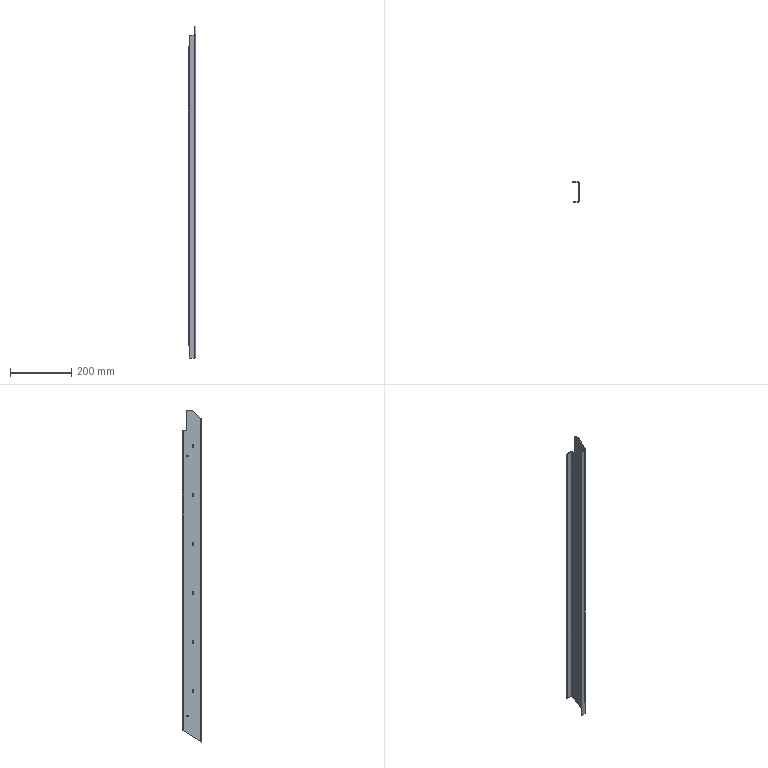Part | NX | features solid 2 | 1 solid | 51 faces | box 23 x 65 x 1085 mm | volume 209039 mm3 | plane 40 | cylinder 8 | spline 3 | commonest cylinder face diameters 4.6 x4 4 x2 8 x2